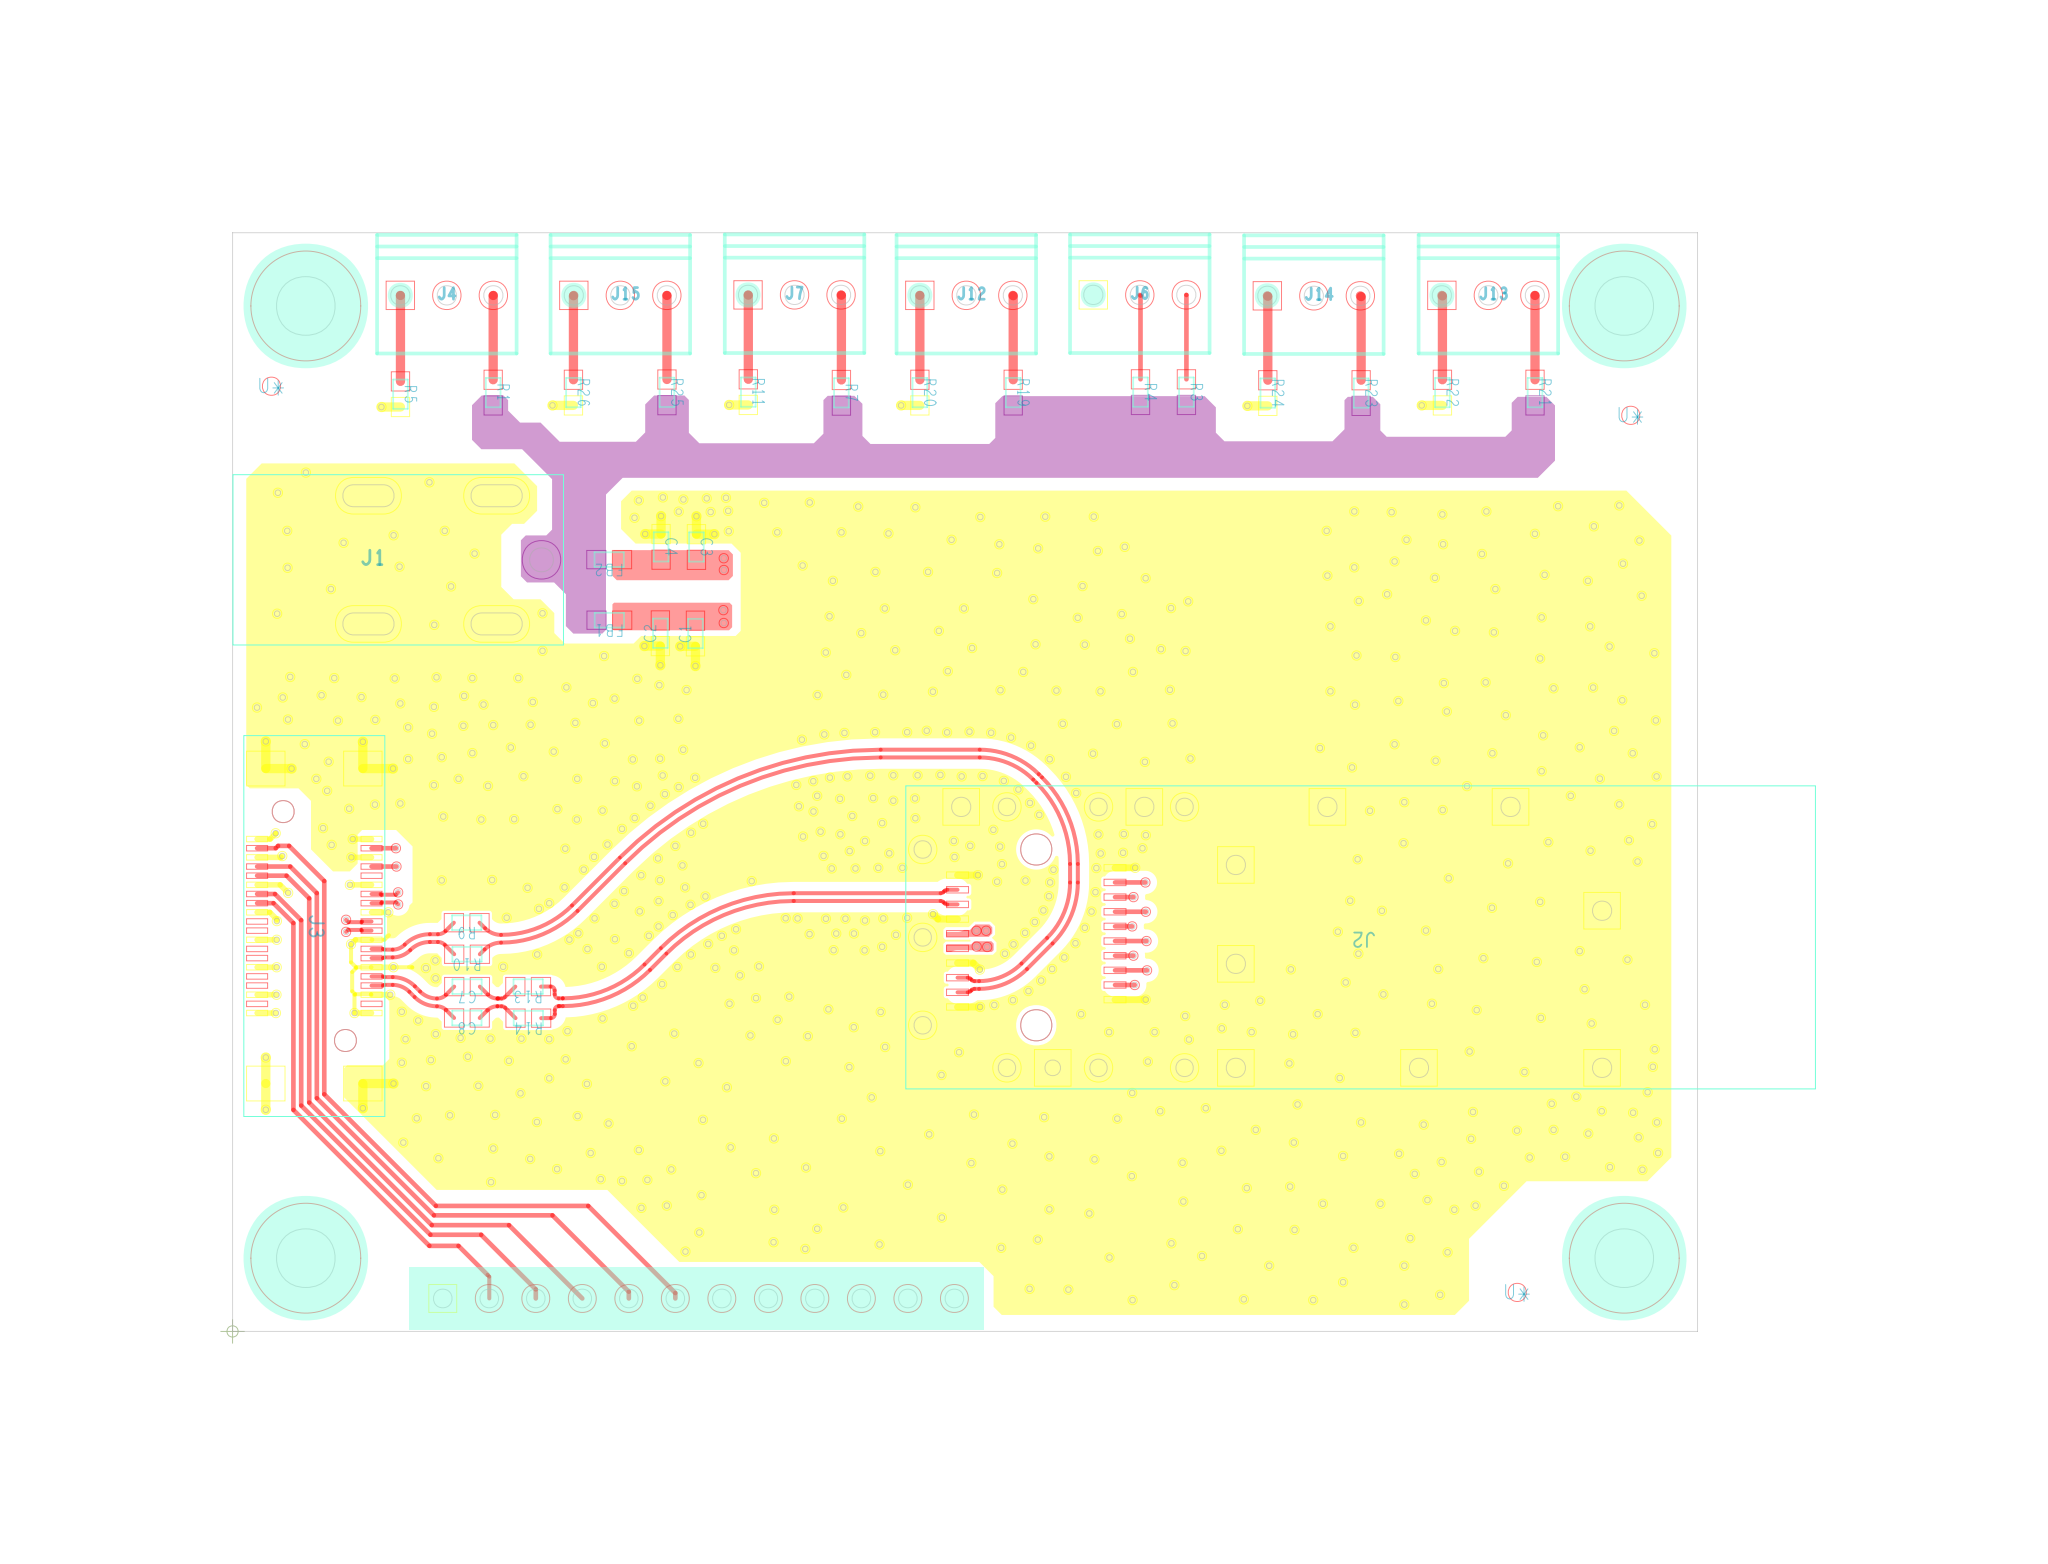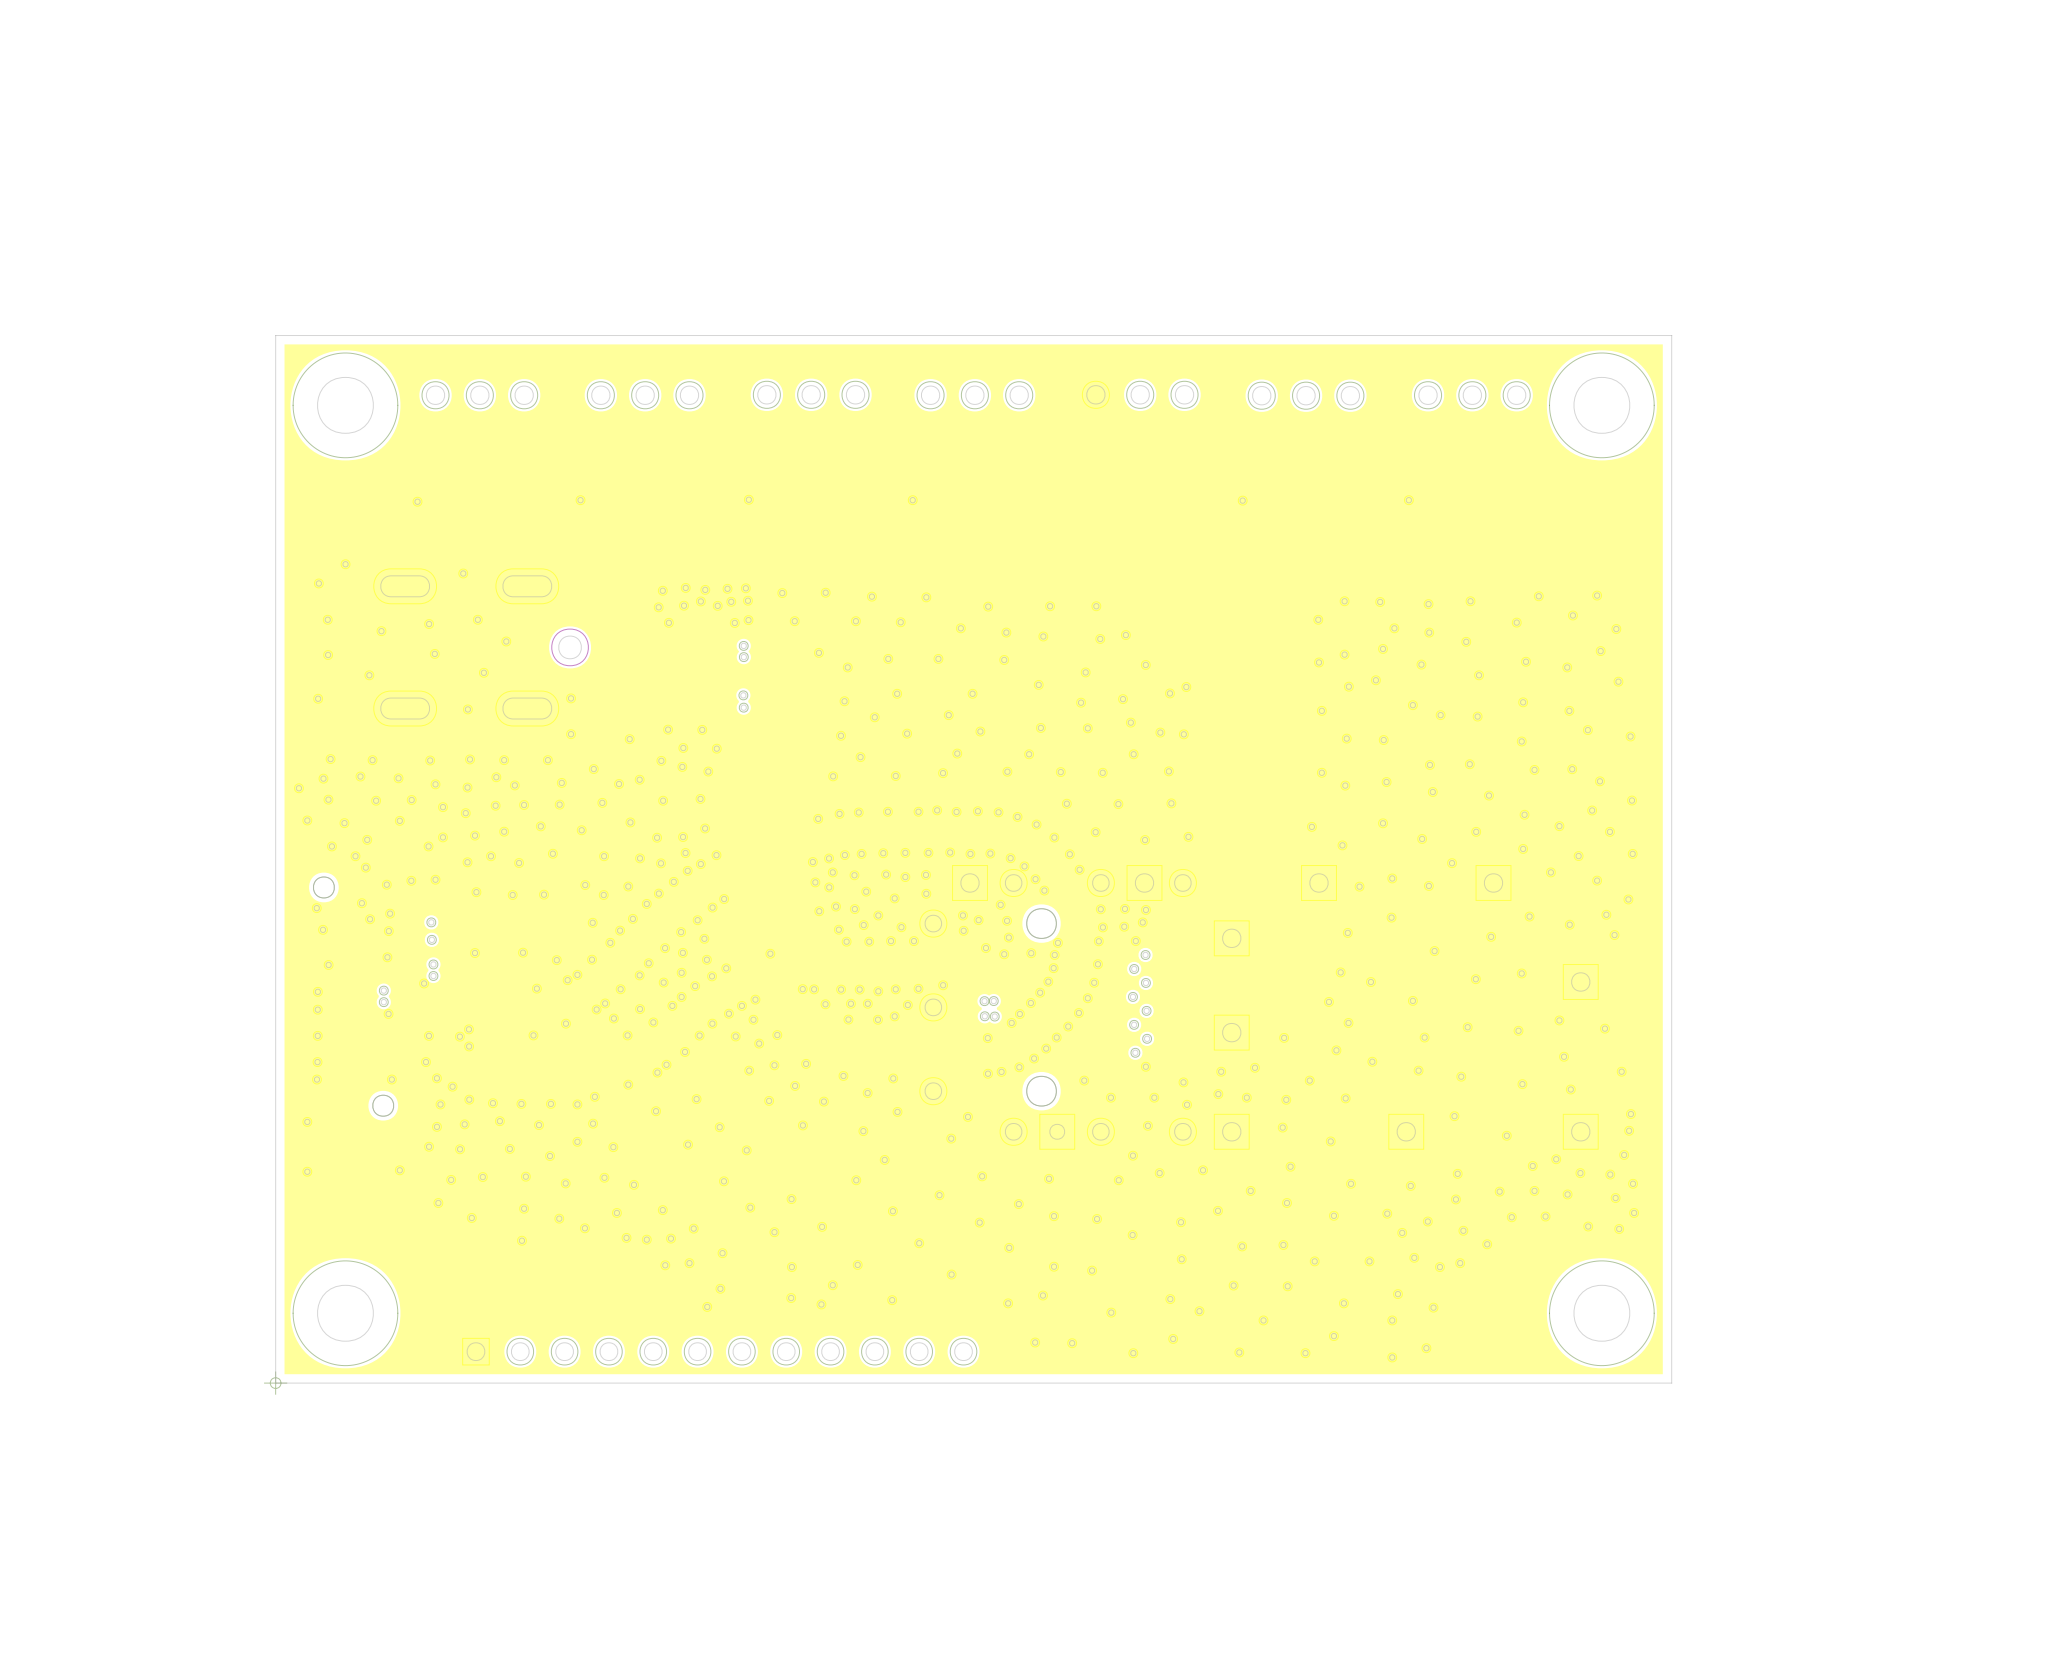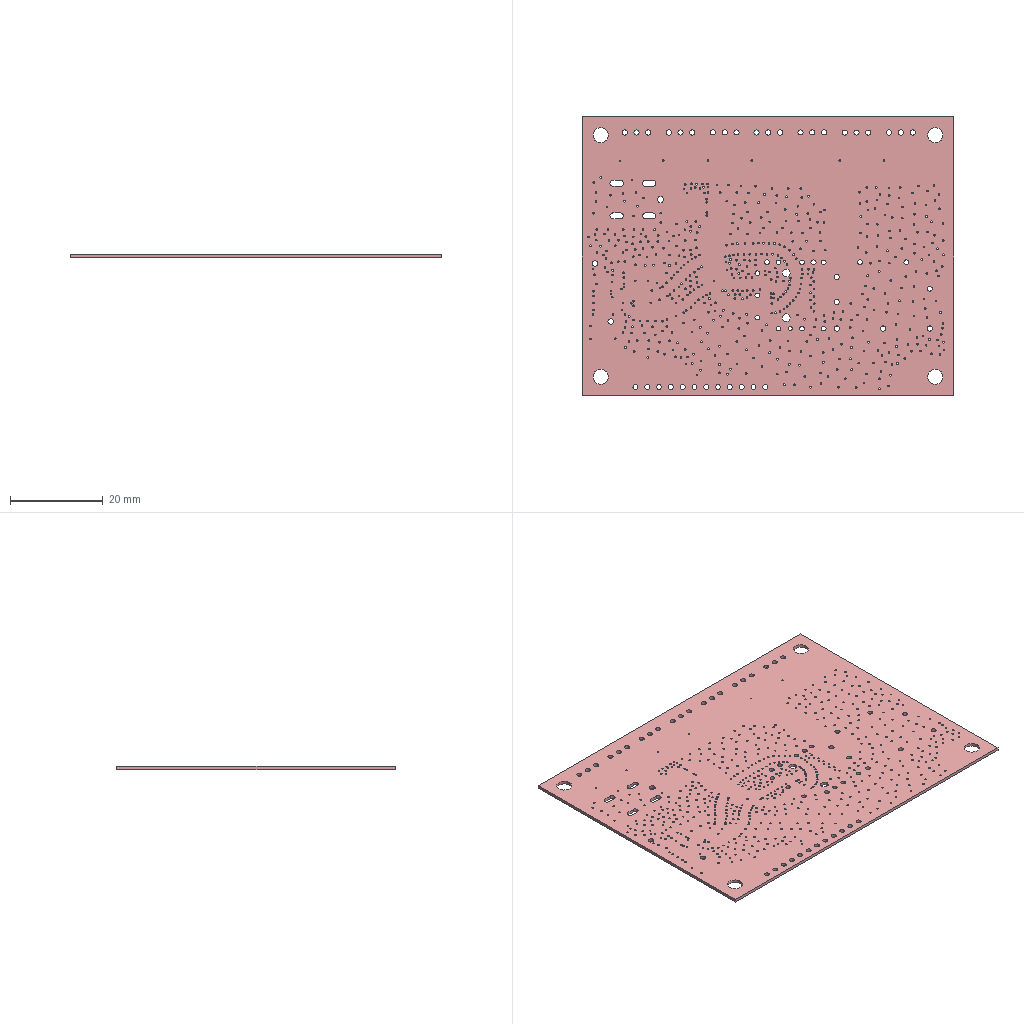Circuit board layout | Cadence Allegro | box 80 x 60 x 0.7 mm
Layer stack:
# Cadence Allegro layer stack of  (unit mm; from the constraint file cross-section; dielectric type: 0 not recorded (Allegro does not mark core vs prepreg), 3 surface material)
index,name,kind,layer,copper_thickness_mm,dielectric_type,dielectric_thickness_mm,dielectric_material,dielectric_constant
0,Top Surface,other,,,,,,
1,TOP,copper,TOP,0.0305,,,,
2,Dielectric1,dielectric,,,0,0.2032,FR-4,4.5
3,GND2,copper,GND2,0.0305,,,,
4,Dielectric2,dielectric,,,0,0.2032,FR-4,4.5
5,GND3,copper,GND3,0.0305,,,,
6,Dielectric3,dielectric,,,0,0.2032,FR-4,4.5
7,BOTTOM,copper,BOTTOM,0.0305,,,,
8,Bottom Surface,other,,,,,,
# drill layer pairs: low layer,high layer
drill_pair,TOP,BOTTOM
Part placement:
REFDES,COMP_VALUE,SYM_NAME,SYM_X,SYM_Y,SYM_ROTATE,SYM_MIRROR
C1,0.1uF,0603,995.220,1500.492,90.000,NO
C2,10uF,0603,919.783,1501.059,90.000,NO
C3,0.1uF,0603,997.327,1686.492,270.000,NO
C4,10uF,0603,921.315,1686.780,270.000,NO
C7,0.1uF,0603,504.130,741.378,180.000,NO
C8,0.1uF,0603,503.831,673.898,180.000,NO
FB1,BLM18KG300TN1D,0603,810.118,1529.138,180.000,NO
FB2,BLM18KG300TN1D,0603,809.728,1659.392,180.000,NO
J1,DC084B,PWR5P_167X80_H78,302.020,1658.906,0.000,NO
J2,SFP_Plus_20p,SFP_CAGE40P_490X161_H91,2433.071,847.193,180.000,NO
J3,IMSA-10143B-40Y902,BTB2X20P_205X74_05_H890_M,175.783,871.551,270.000,NO
J4,header_2.54_3,003_HDR_KK,460.697,2227.520,0.000,NO
J6,header_2.54_3,003_HDR_KK,1950.559,2228.520,0.000,NO
J7,header_2.54_3,003_HDR_KK,1208.256,2228.520,0.000,NO
J9,Header_1_12,DIP1X12,1001.949,70.870,90.000,NO
J12,header_2.54_3,003_HDR_KK,1577.559,2227.520,0.000,NO
J13,header_2.54_3,003_HDR_KK,2699.941,2227.520,0.000,NO
J14,header_2.54_3,003_HDR_KK,2324.736,2226.520,0.000,NO
J15,header_2.54_3,003_HDR_KK,833.689,2227.520,0.000,NO
R1,4.7K,0603,560.335,2018.457,270.000,NO
R3,4.7K,0603,2050.776,2019.457,270.000,NO
R4,4.7K,0603,1952.055,2019.457,270.000,NO
R5,49.9K,0603,361.000,2015.000,270.000,NO
R7,4.7K,0603,1309.000,2018.000,270.000,NO
R9,0,0603,503.417,878.783,180.000,NO
R10,0,0603,504.083,810.921,180.000,NO
R11,49.9K,0603,1108.843,2019.457,270.000,NO
R13,0,0603,635.528,741.394,180.000,NO
R14,0,0603,635.961,673.539,180.000,NO
R19,4.7K,0603,1678.366,2018.461,270.000,NO
R20,4.7K,0603,1477.697,2018.457,270.000,NO
R21,4.7K,0603,2800.232,2018.457,270.000,NO
R22,4.7K,0603,2601.177,2018.457,270.000,NO
R23,4.7K,0603,2426.417,2017.457,270.000,NO
R24,4.7K,0603,2225.752,2017.457,270.000,NO
R25,4.7K,0603,933.940,2019.004,270.000,NO
R26,4.7K,0603,732.882,2018.457,270.000,NO
Pad and via stacks, first 115 of 285 lines:
# Allegro (Cadence) via spans and padstacks; design units: ("mils" 3 1000)
# via spans: padstack,start_layer,end_layer,net_example,count
VIA12X20,ETCH/TOP,ETCH/BOTTOM,GND,634
# Allegro padstack definitions: name,start_layer,end_layer,drill,plating,holeType,type
PAD19,"ETCH/TOP","ETCH/TOP",0.0,"NON_PLATED","none","smd"
PAD13,"ETCH/TOP","ETCH/TOP",0.0,"NON_PLATED","none","smd"
PAD12,"ETCH/TOP","ETCH/TOP",0.0,"NON_PLATED","none","smd"
PAD17,"ETCH/TOP","ETCH/TOP",0.0,"NON_PLATED","none","smd"
PAD15,"ETCH/TOP","ETCH/TOP",0.0,"NON_PLATED","none","smd"
PAD16,"ETCH/TOP","ETCH/TOP",0.0,"NON_PLATED","none","smd"
PAD1,"ETCH/TOP","ETCH/TOP",0.0,"NON_PLATED","none","smd"
PAD46,"ETCH/TOP","ETCH/TOP",0.0,"NON_PLATED","none","smd"
PAD44,"ETCH/TOP","ETCH/TOP",0.0,"NON_PLATED","none","smd"
PAD8,"ETCH/TOP","ETCH/TOP",0.0,"NON_PLATED","none","smd"
PAD5,"ETCH/TOP","ETCH/TOP",0.0,"NON_PLATED","none","smd"
PAD9,"ETCH/TOP","ETCH/TOP",0.0,"NON_PLATED","none","smd"
PAD10,"ETCH/TOP","ETCH/TOP",0.0,"NON_PLATED","none","smd"
PAD25,"ETCH/TOP","ETCH/TOP",0.0,"NON_PLATED","none","smd"
PAD4,"ETCH/TOP","ETCH/TOP",0.0,"NON_PLATED","none","smd"
PAD7,"ETCH/TOP","ETCH/TOP",0.0,"NON_PLATED","none","smd"
PAD6,"ETCH/TOP","ETCH/TOP",0.0,"NON_PLATED","none","smd"
PAD3,"ETCH/TOP","ETCH/TOP",0.0,"NON_PLATED","none","smd"
PAD31,"ETCH/TOP","ETCH/TOP",0.0,"NON_PLATED","none","smd"
PAD22,"ETCH/TOP","ETCH/TOP",0.0,"NON_PLATED","none","smd"
PAD41,"ETCH/TOP","ETCH/TOP",0.0,"NON_PLATED","none","smd"
PAD42,"ETCH/TOP","ETCH/TOP",0.0,"NON_PLATED","none","smd"
PAD43,"ETCH/TOP","ETCH/TOP",0.0,"NON_PLATED","none","smd"
PAD45,"ETCH/TOP","ETCH/TOP",0.0,"NON_PLATED","none","smd"
PAD2,"ETCH/TOP","ETCH/TOP",0.0,"NON_PLATED","none","smd"
PAD14,"ETCH/TOP","ETCH/TOP",0.0,"NON_PLATED","none","smd"
PAD21,"ETCH/TOP","ETCH/TOP",0.0,"NON_PLATED","none","smd"
PAD28,"ETCH/TOP","ETCH/TOP",0.0,"NON_PLATED","none","smd"
PAD26,"ETCH/TOP","ETCH/TOP",0.0,"NON_PLATED","none","smd"
PAD27,"ETCH/TOP","ETCH/TOP",0.0,"NON_PLATED","none","smd"
PAD18,"ETCH/TOP","ETCH/TOP",0.0,"NON_PLATED","none","smd"
PAD29,"ETCH/TOP","ETCH/TOP",0.0,"NON_PLATED","none","smd"
PAD20,"ETCH/TOP","ETCH/TOP",0.0,"NON_PLATED","none","smd"
PAD39,"ETCH/TOP","ETCH/TOP",0.0,"NON_PLATED","none","smd"
PAD40,"ETCH/TOP","ETCH/TOP",0.0,"NON_PLATED","none","smd"
PAD30,"ETCH/TOP","ETCH/TOP",0.0,"NON_PLATED","none","smd"
PAD48,"ETCH/TOP","ETCH/TOP",0.0,"NON_PLATED","none","smd"
PAD47,"ETCH/TOP","ETCH/TOP",0.0,"NON_PLATED","none","smd"
PAD49,"ETCH/TOP","ETCH/TOP",0.0,"NON_PLATED","none","smd"
PAD50,"ETCH/TOP","ETCH/TOP",0.0,"NON_PLATED","none","smd"
PAD53,"ETCH/TOP","ETCH/TOP",0.0,"NON_PLATED","none","smd"
F45,"ETCH/TOP","ETCH/TOP",0.0,"NON_PLATED","none","smd"
R88X76,"ETCH/TOP","ETCH/TOP",0.0,"PLATED","none","smd"
R127X121,"ETCH/TOP","ETCH/TOP",0.0,"PLATED","none","smd"
R127X152,"ETCH/TOP","ETCH/TOP",0.0,"NON_PLATED","none","smd"
R14X25,"ETCH/TOP","ETCH/TOP",0.0,"NON_PLATED","none","smd"
R165X317,"ETCH/TOP","ETCH/TOP",0.0,"NON_PLATED","none","smd"
R259X218,"ETCH/TOP","ETCH/TOP",0.0,"NON_PLATED","none","smd"
R70X22,"ETCH/TOP","ETCH/TOP",0.0,"NON_PLATED","none","smd"
R75X85,"ETCH/TOP","ETCH/TOP",0.0,"NON_PLATED","none","smd"
Y5,"ETCH/TOP","ETCH/TOP",0.0,"NON_PLATED","none","smd"
R16X30,"ETCH/TOP","ETCH/TOP",0.0,"NON_PLATED","none","smd"
F62X58,"ETCH/TOP","ETCH/TOP",0.0,"PLATED","none","smd"
R15X28,"ETCH/TOP","ETCH/TOP",0.0,"NON_PLATED","none","smd"
R195X280,"ETCH/TOP","ETCH/TOP",0.0,"NON_PLATED","none","smd"
R45X200,"ETCH/TOP","ETCH/TOP",0.0,"NON_PLATED","none","smd"
R50X30,"ETCH/TOP","ETCH/TOP",0.0,"NON_PLATED","none","smd"
R127X120,"ETCH/TOP","ETCH/TOP",0.0,"NON_PLATED","none","smd"
R31X24,"ETCH/TOP","ETCH/TOP",0.0,"NON_PLATED","none","smd"
R215X60,"ETCH/TOP","ETCH/TOP",0.0,"NON_PLATED","none","smd"
S17,"ETCH/TOP","ETCH/TOP",0.0,"NON_PLATED","none","smd"
R23X25,"ETCH/TOP","ETCH/TOP",0.0,"NON_PLATED","none","smd"
R19X32,"ETCH/TOP","ETCH/TOP",0.0,"NON_PLATED","none","smd"
R61X15,"ETCH/TOP","ETCH/TOP",0.0,"NON_PLATED","none","smd"
R45X150,"ETCH/TOP","ETCH/TOP",0.0,"NON_PLATED","none","smd"
R12X8,"ETCH/TOP","ETCH/TOP",0.0,"NON_PLATED","none","smd"
R91X127,"ETCH/TOP","ETCH/TOP",0.0,"NON_PLATED","none","smd"
S91,"ETCH/TOP","ETCH/TOP",0.0,"NON_PLATED","none","smd"
R55X99,"ETCH/TOP","ETCH/TOP",0.0,"NON_PLATED","none","smd"
R299X199,"ETCH/TOP","ETCH/TOP",0.0,"NON_PLATED","none","smd"
R114X165,"ETCH/TOP","ETCH/TOP",0.0,"NON_PLATED","none","smd"
R60X90,"ETCH/TOP","ETCH/TOP",0.0,"NON_PLATED","none","smd"
R6X10,"ETCH/TOP","ETCH/TOP",0.0,"NON_PLATED","none","smd"
Y10,"ETCH/TOP","ETCH/TOP",0.0,"NON_PLATED","none","smd"
R114X74,"ETCH/TOP","ETCH/TOP",0.0,"NON_PLATED","none","smd"
R30X130,"ETCH/TOP","ETCH/TOP",0.0,"PLATED","none","smd"
R50X127,"ETCH/TOP","ETCH/TOP",0.0,"NON_PLATED","none","smd"
R18X20,"ETCH/TOP","ETCH/TOP",0.0,"NON_PLATED","none","smd"
R60X71,"ETCH/TOP","ETCH/TOP",0.0,"NON_PLATED","none","smd"
R48X71,"ETCH/TOP","ETCH/TOP",0.0,"NON_PLATED","none","smd"
R80X30,"ETCH/TOP","ETCH/TOP",0.0,"PLATED","none","smd"
FLASH_0,"ETCH/TOP","ETCH/TOP",0.0,"PLATED","none","smd"
Y3,"ETCH/TOP","ETCH/TOP",0.0,"PLATED","none","smd"
R170X25,"ETCH/TOP","ETCH/TOP",0.0,"PLATED","none","smd"
R70X25,"ETCH/TOP","ETCH/TOP",0.0,"PLATED","none","smd"
R43X14,"ETCH/TOP","ETCH/TOP",0.0,"PLATED","none","smd"
R33X10,"ETCH/TOP","ETCH/TOP",0.0,"PLATED","none","smd"
R636X23,"ETCH/TOP","ETCH/TOP",0.0,"PLATED","none","smd"
R155X35,"ETCH/TOP","ETCH/TOP",0.0,"PLATED","none","smd"
R60X20,"ETCH/TOP","ETCH/TOP",0.0,"PLATED","none","smd"
R120X70,"ETCH/TOP","ETCH/TOP",0.0,"PLATED","none","smd"
SMD0_45R,"ETCH/TOP","ETCH/TOP",0.0,"PLATED","none","smd"
Y42,"ETCH/TOP","ETCH/TOP",0.0,"PLATED","none","smd"
R85X65,"ETCH/TOP","ETCH/TOP",0.0,"PLATED","none","smd"
Y30,"ETCH/TOP","ETCH/TOP",0.0,"PLATED","none","smd"
R53X20,"ETCH/TOP","ETCH/TOP",0.0,"PLATED","none","smd"
R55X40,"ETCH/TOP","ETCH/TOP",0.0,"PLATED","none","smd"
R155X25,"ETCH/TOP","ETCH/TOP",0.0,"PLATED","none","smd"
F17X17,"ETCH/TOP","ETCH/TOP",0.0,"PLATED","none","smd"
F89X32,"ETCH/TOP","ETCH/TOP",0.0,"PLATED","none","smd"
R8X2,"ETCH/TOP","ETCH/TOP",0.0,"PLATED","none","smd"
SMD40X20,"ETCH/TOP","ETCH/TOP",0.0,"PLATED","none","smd"
R340X185,"ETCH/TOP","ETCH/TOP",0.0,"PLATED","none","smd"
R27X10,"ETCH/TOP","ETCH/TOP",0.0,"PLATED","none","smd"
R22X11,"ETCH/TOP","ETCH/TOP",0.0,"PLATED","none","smd"
R32X36,"ETCH/TOP","ETCH/TOP",0.0,"PLATED","none","smd"
S21X20,"ETCH/TOP","ETCH/TOP",0.0,"PLATED","none","smd"
R13X10,"ETCH/TOP","ETCH/TOP",0.0,"PLATED","none","smd"
R75X28,"ETCH/TOP","ETCH/TOP",0.0,"PLATED","none","smd"
R25X15,"ETCH/TOP","ETCH/TOP",0.0,"NON_PLATED","none","smd"
C0_5,"ETCH/TOP","ETCH/TOP",0.0,"PLATED","none","smd"
Design rules, without the lines most boards share, first 15 of 34 lines:
# Cadence Allegro design rules of  (from the Constraint Manager export constraints.dcfx, design unit mil; typed fields in mm)
# columns: name | kind | enabled | priority | scope1 | scope2 | descriptor | typed fields (field=value)
# Allegro precedence (priority 1 wins): 1 Region class-to-class, 2 Region class, 3 Region, 4 class-to-class, 5 DiffPair/Bus/NetGroup override, 6 NetClass, 7 constraint set (CSet) default
# per-layer values are written LAYER=value in the descriptor and LAYER:mm in the typed field; a maximum of 0 means no limit set
# --- net classes (and buses / net groups) ---
PHY_R | NetClass | enabled | 6 | no members | All | Net Class (members: 0) |
PHY_T | NetClass | enabled | 6 | no members | All | Net Class (members: 0) |
DDR3_A | NetClass | enabled | 6 | no members | All | Net Class (members: 0) |
DDR3_DQH1 | NetClass | enabled | 6 | no members | All | Net Class (members: 0) |
DDR3_DQL1 | NetClass | enabled | 6 | no members | All | Net Class (members: 0) |
DDR3_DQH0 | NetClass | enabled | 6 | no members | All | Net Class (members: 0) |
DDR3_DQL0 | NetClass | enabled | 6 | no members | All | Net Class (members: 0) |
# --- track widths, neck and differential-pair gap (physical constraint sets) ---
DEFAULT | PhysicalCSet | enabled | 7 | Design default | All | Physical Constraint (Min Line Width=8.68mil) (Max Line Width=0mil) (Min Neck Width=8.68mil) (Max Neck Length=0mil) (DiffPair Primary Gap=8mil) (DiffPair Neck Gap=0mil) (DiffPair Min Space=0mil) (DiffPair Coupled +Tol=0mil) (DiffPair Coupled -Tol=0mil) (Min BB Via Stagger=5mil) (Max BB Via Stagger=0mil) (T-junctions=ANYWHERE) (Pad-pad direct connect=ALL_ALLOWED) (Allowed vias=VIA12X20) | min_line_width=0.2205 min_neck_width=0.2205 min_bvia_stagger=0.127 max_bvia_stagger=0 ts_allowed=ANYWHERE diffp_primary_gap=0.2032 diffp_neck_gap=0 max_line_width=0 maximum_neck_length=0 pad_pad_direct_connect=ALL_ALLOWED allow_on_etch_subclass=TRUE diffp_coupled_plus=0 diffp_coupled_minus=0 diffp_min_space=0 vias=VIA12X20
# --- clearances: line / pad / via / shape / hole (spacing constraint sets) ---